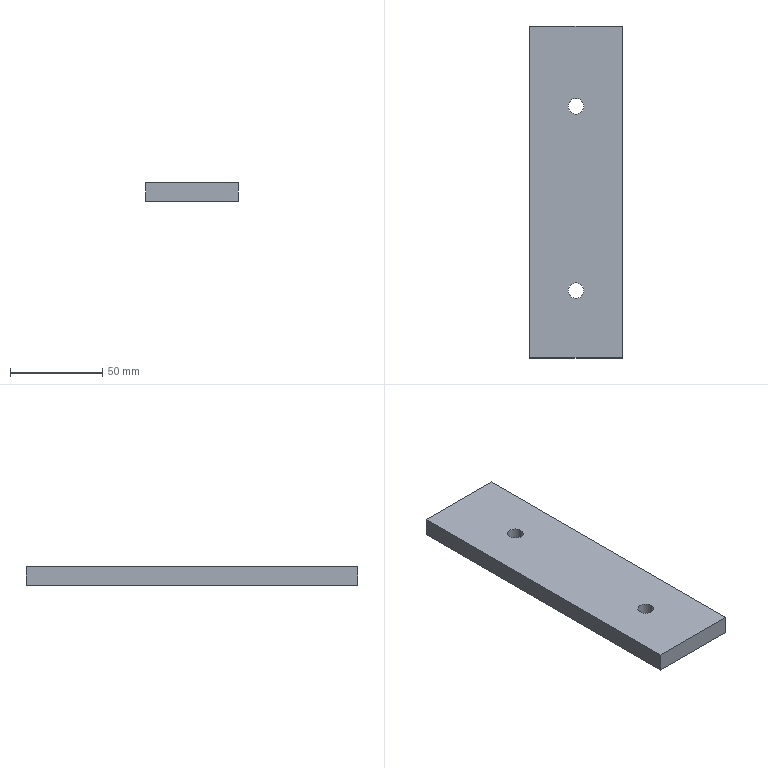Part | SolidWorks | features BaseBody 1, ICE 1 | 1 solid | 10 faces | box 50 x 180 x 10 mm | volume 88865 mm3 | plane 6 | cylinder 4 | commonest cylinder face diameters 8.5 x4
STEP:
#1=CARTESIAN_POINT('',(4.25,46.5,0.));
#2=VERTEX_POINT('',#1);
#3=CARTESIAN_POINT('',(-4.25,46.5,0.));
#4=VERTEX_POINT('',#3);
#5=CARTESIAN_POINT('',(0.,46.5,0.));
#6=DIRECTION('',(0.,0.,-1.));
#7=DIRECTION('',(1.,0.,0.));
#8=AXIS2_PLACEMENT_3D('',#5,#6,#7);
#9=CIRCLE('',#8,4.25);
#10=EDGE_CURVE('',#2,#4,#9,.T.);
#11=ORIENTED_EDGE('',*,*,#10,.T.);
#12=CARTESIAN_POINT('',(-4.25,46.5,10.));
#13=VERTEX_POINT('',#12);
#14=CARTESIAN_POINT('',(-4.25,46.5,-0.001));
#15=DIRECTION('',(0.,0.,1.));
#16=VECTOR('',#15,1000.);
#17=LINE('',#14,#16);
#18=EDGE_CURVE('',#4,#13,#17,.T.);
#19=ORIENTED_EDGE('',*,*,#18,.T.);
#20=CARTESIAN_POINT('',(4.25,46.5,10.));
#21=VERTEX_POINT('',#20);
#22=CARTESIAN_POINT('',(0.,46.5,10.));
#23=DIRECTION('',(0.,0.,1.));
#24=DIRECTION('',(1.,0.,0.));
#25=AXIS2_PLACEMENT_3D('',#22,#23,#24);
#26=CIRCLE('',#25,4.25);
#27=EDGE_CURVE('',#13,#21,#26,.T.);
#28=ORIENTED_EDGE('',*,*,#27,.T.);
#29=CARTESIAN_POINT('',(4.25,46.5,-0.001));
#30=DIRECTION('',(0.,0.,1.));
#31=VECTOR('',#30,1000.);
#32=LINE('',#29,#31);
#33=EDGE_CURVE('',#2,#21,#32,.T.);
#34=ORIENTED_EDGE('',*,*,#33,.F.);
#35=EDGE_LOOP('',(#11,#19,#28,#34));
#36=FACE_OUTER_BOUND('',#35,.T.);
#37=CARTESIAN_POINT('',(0.,46.5,-0.001));
#38=DIRECTION('',(0.,0.,1.));
#39=DIRECTION('',(1.,0.,0.));
#40=AXIS2_PLACEMENT_3D('',#37,#38,#39);
#41=CYLINDRICAL_SURFACE('',#40,4.25);
#42=ADVANCED_FACE('',(#36),#41,.F.);
#43=CARTESIAN_POINT('',(4.25,-53.5,0.));
#44=VERTEX_POINT('',#43);
#45=CARTESIAN_POINT('',(-4.25,-53.5,0.));
#46=VERTEX_POINT('',#45);
#47=CARTESIAN_POINT('',(0.,-53.5,0.));
#48=DIRECTION('',(0.,0.,-1.));
#49=DIRECTION('',(1.,0.,0.));
#50=AXIS2_PLACEMENT_3D('',#47,#48,#49);
#51=CIRCLE('',#50,4.25);
#52=EDGE_CURVE('',#44,#46,#51,.T.);
#53=ORIENTED_EDGE('',*,*,#52,.T.);
#54=CARTESIAN_POINT('',(-4.25,-53.5,10.));
#55=VERTEX_POINT('',#54);
#56=CARTESIAN_POINT('',(-4.25,-53.5,-0.001));
#57=DIRECTION('',(0.,0.,1.));
#58=VECTOR('',#57,1000.);
#59=LINE('',#56,#58);
#60=EDGE_CURVE('',#46,#55,#59,.T.);
#61=ORIENTED_EDGE('',*,*,#60,.T.);
#62=CARTESIAN_POINT('',(4.25,-53.5,10.));
#63=VERTEX_POINT('',#62);
#64=CARTESIAN_POINT('',(0.,-53.5,10.));
#65=DIRECTION('',(0.,0.,1.));
#66=DIRECTION('',(1.,0.,0.));
#67=AXIS2_PLACEMENT_3D('',#64,#65,#66);
#68=CIRCLE('',#67,4.25);
#69=EDGE_CURVE('',#55,#63,#68,.T.);
#70=ORIENTED_EDGE('',*,*,#69,.T.);
#71=CARTESIAN_POINT('',(4.25,-53.5,-0.001));
#72=DIRECTION('',(0.,0.,1.));
#73=VECTOR('',#72,1000.);
#74=LINE('',#71,#73);
#75=EDGE_CURVE('',#44,#63,#74,.T.);
#76=ORIENTED_EDGE('',*,*,#75,.F.);
#77=EDGE_LOOP('',(#53,#61,#70,#76));
#78=FACE_OUTER_BOUND('',#77,.T.);
#79=CARTESIAN_POINT('',(0.,-53.5,-0.001));
#80=DIRECTION('',(0.,0.,1.));
#81=DIRECTION('',(1.,0.,0.));
#82=AXIS2_PLACEMENT_3D('',#79,#80,#81);
#83=CYLINDRICAL_SURFACE('',#82,4.25);
#84=ADVANCED_FACE('',(#78),#83,.F.);
#85=ORIENTED_EDGE('',*,*,#10,.F.);
#86=CARTESIAN_POINT('',(0.,46.5,0.));
#87=DIRECTION('',(0.,0.,-1.));
#88=DIRECTION('',(1.,0.,0.));
#89=AXIS2_PLACEMENT_3D('',#86,#87,#88);
#90=CIRCLE('',#89,4.25);
#91=EDGE_CURVE('',#4,#2,#90,.T.);
#92=ORIENTED_EDGE('',*,*,#91,.F.);
#93=EDGE_LOOP('',(#85,#92));
#94=FACE_BOUND('',#93,.T.);
#95=ORIENTED_EDGE('',*,*,#52,.F.);
#96=CARTESIAN_POINT('',(0.,-53.5,0.));
#97=DIRECTION('',(0.,0.,-1.));
#98=DIRECTION('',(1.,0.,0.));
#99=AXIS2_PLACEMENT_3D('',#96,#97,#98);
#100=CIRCLE('',#99,4.25);
#101=EDGE_CURVE('',#46,#44,#100,.T.);
#102=ORIENTED_EDGE('',*,*,#101,.F.);
#103=EDGE_LOOP('',(#95,#102));
#104=FACE_BOUND('',#103,.T.);
#105=CARTESIAN_POINT('',(25.,-90.,0.));
#106=VERTEX_POINT('',#105);
#107=CARTESIAN_POINT('',(25.,90.,0.));
#108=VERTEX_POINT('',#107);
#109=CARTESIAN_POINT('',(25.,90.,0.));
#110=DIRECTION('',(0.,1.,0.));
#111=VECTOR('',#110,1000.);
#112=LINE('',#109,#111);
#113=EDGE_CURVE('',#106,#108,#112,.T.);
#114=ORIENTED_EDGE('',*,*,#113,.F.);
#115=CARTESIAN_POINT('',(-25.,-90.,0.));
#116=VERTEX_POINT('',#115);
#117=CARTESIAN_POINT('',(-25.,-90.,0.));
#118=DIRECTION('',(1.,0.,0.));
#119=VECTOR('',#118,1000.);
#120=LINE('',#117,#119);
#121=EDGE_CURVE('',#116,#106,#120,.T.);
#122=ORIENTED_EDGE('',*,*,#121,.F.);
#123=CARTESIAN_POINT('',(-25.,90.,0.));
#124=VERTEX_POINT('',#123);
#125=CARTESIAN_POINT('',(-25.,90.,0.));
#126=DIRECTION('',(0.,-1.,0.));
#127=VECTOR('',#126,1000.);
#128=LINE('',#125,#127);
#129=EDGE_CURVE('',#124,#116,#128,.T.);
#130=ORIENTED_EDGE('',*,*,#129,.F.);
#131=CARTESIAN_POINT('',(-25.,90.,0.));
#132=DIRECTION('',(-1.,0.,0.));
#133=VECTOR('',#132,1000.);
#134=LINE('',#131,#133);
#135=EDGE_CURVE('',#108,#124,#134,.T.);
#136=ORIENTED_EDGE('',*,*,#135,.F.);
#137=EDGE_LOOP('',(#114,#122,#130,#136));
#138=FACE_OUTER_BOUND('',#137,.T.);
#139=CARTESIAN_POINT('',(0.,0.,0.));
#140=DIRECTION('',(0.,0.,1.));
#141=DIRECTION('',(1.,0.,0.));
#142=AXIS2_PLACEMENT_3D('',#139,#140,#141);
#143=PLANE('',#142);
#144=ADVANCED_FACE('',(#94,#104,#138),#143,.F.);
#145=CARTESIAN_POINT('',(0.,46.5,10.));
#146=DIRECTION('',(0.,0.,1.));
#147=DIRECTION('',(1.,0.,0.));
#148=AXIS2_PLACEMENT_3D('',#145,#146,#147);
#149=CIRCLE('',#148,4.25);
#150=EDGE_CURVE('',#21,#13,#149,.T.);
#151=ORIENTED_EDGE('',*,*,#150,.F.);
#152=ORIENTED_EDGE('',*,*,#27,.F.);
#153=EDGE_LOOP('',(#151,#152));
#154=FACE_BOUND('',#153,.T.);
#155=CARTESIAN_POINT('',(0.,-53.5,10.));
#156=DIRECTION('',(0.,0.,1.));
#157=DIRECTION('',(1.,0.,0.));
#158=AXIS2_PLACEMENT_3D('',#155,#156,#157);
#159=CIRCLE('',#158,4.25);
#160=EDGE_CURVE('',#63,#55,#159,.T.);
#161=ORIENTED_EDGE('',*,*,#160,.F.);
#162=ORIENTED_EDGE('',*,*,#69,.F.);
#163=EDGE_LOOP('',(#161,#162));
#164=FACE_BOUND('',#163,.T.);
#165=CARTESIAN_POINT('',(25.,-90.,10.));
#166=VERTEX_POINT('',#165);
#167=CARTESIAN_POINT('',(25.,90.,10.));
#168=VERTEX_POINT('',#167);
#169=CARTESIAN_POINT('',(25.,90.,10.));
#170=DIRECTION('',(0.,1.,0.));
#171=VECTOR('',#170,1000.);
#172=LINE('',#169,#171);
#173=EDGE_CURVE('',#166,#168,#172,.T.);
#174=ORIENTED_EDGE('',*,*,#173,.T.);
#175=CARTESIAN_POINT('',(-25.,90.,10.));
#176=VERTEX_POINT('',#175);
#177=CARTESIAN_POINT('',(-25.,90.,10.));
#178=DIRECTION('',(-1.,0.,0.));
#179=VECTOR('',#178,1000.);
#180=LINE('',#177,#179);
#181=EDGE_CURVE('',#168,#176,#180,.T.);
#182=ORIENTED_EDGE('',*,*,#181,.T.);
#183=CARTESIAN_POINT('',(-25.,-90.,10.));
#184=VERTEX_POINT('',#183);
#185=CARTESIAN_POINT('',(-25.,90.,10.));
#186=DIRECTION('',(0.,-1.,0.));
#187=VECTOR('',#186,1000.);
#188=LINE('',#185,#187);
#189=EDGE_CURVE('',#176,#184,#188,.T.);
#190=ORIENTED_EDGE('',*,*,#189,.T.);
#191=CARTESIAN_POINT('',(-25.,-90.,10.));
#192=DIRECTION('',(1.,0.,0.));
#193=VECTOR('',#192,1000.);
#194=LINE('',#191,#193);
#195=EDGE_CURVE('',#184,#166,#194,.T.);
#196=ORIENTED_EDGE('',*,*,#195,.T.);
#197=EDGE_LOOP('',(#174,#182,#190,#196));
#198=FACE_OUTER_BOUND('',#197,.T.);
#199=CARTESIAN_POINT('',(0.,0.,10.));
#200=DIRECTION('',(0.,0.,1.));
#201=DIRECTION('',(1.,0.,0.));
#202=AXIS2_PLACEMENT_3D('',#199,#200,#201);
#203=PLANE('',#202);
#204=ADVANCED_FACE('',(#154,#164,#198),#203,.T.);
#205=ORIENTED_EDGE('',*,*,#121,.T.);
#206=CARTESIAN_POINT('',(25.,-90.,10.));
#207=DIRECTION('',(0.,0.,-1.));
#208=VECTOR('',#207,1000.);
#209=LINE('',#206,#208);
#210=EDGE_CURVE('',#166,#106,#209,.T.);
#211=ORIENTED_EDGE('',*,*,#210,.F.);
#212=ORIENTED_EDGE('',*,*,#195,.F.);
#213=CARTESIAN_POINT('',(-25.,-90.,10.));
#214=DIRECTION('',(0.,0.,-1.));
#215=VECTOR('',#214,1000.);
#216=LINE('',#213,#215);
#217=EDGE_CURVE('',#184,#116,#216,.T.);
#218=ORIENTED_EDGE('',*,*,#217,.T.);
#219=EDGE_LOOP('',(#205,#211,#212,#218));
#220=FACE_OUTER_BOUND('',#219,.T.);
#221=CARTESIAN_POINT('',(-25.,-90.,10.));
#222=DIRECTION('',(0.,1.,0.));
#223=DIRECTION('',(1.,0.,0.));
#224=AXIS2_PLACEMENT_3D('',#221,#222,#223);
#225=PLANE('',#224);
#226=ADVANCED_FACE('',(#220),#225,.F.);
#227=ORIENTED_EDGE('',*,*,#129,.T.);
#228=ORIENTED_EDGE('',*,*,#217,.F.);
#229=ORIENTED_EDGE('',*,*,#189,.F.);
#230=CARTESIAN_POINT('',(-25.,90.,10.));
#231=DIRECTION('',(0.,0.,-1.));
#232=VECTOR('',#231,1000.);
#233=LINE('',#230,#232);
#234=EDGE_CURVE('',#176,#124,#233,.T.);
#235=ORIENTED_EDGE('',*,*,#234,.T.);
#236=EDGE_LOOP('',(#227,#228,#229,#235));
#237=FACE_OUTER_BOUND('',#236,.T.);
#238=CARTESIAN_POINT('',(-25.,90.,10.));
#239=DIRECTION('',(1.,0.,0.));
#240=DIRECTION('',(0.,1.,0.));
#241=AXIS2_PLACEMENT_3D('',#238,#239,#240);
#242=PLANE('',#241);
#243=ADVANCED_FACE('',(#237),#242,.F.);
#244=ORIENTED_EDGE('',*,*,#135,.T.);
#245=ORIENTED_EDGE('',*,*,#234,.F.);
#246=ORIENTED_EDGE('',*,*,#181,.F.);
#247=CARTESIAN_POINT('',(25.,90.,10.));
#248=DIRECTION('',(0.,0.,-1.));
#249=VECTOR('',#248,1000.);
#250=LINE('',#247,#249);
#251=EDGE_CURVE('',#168,#108,#250,.T.);
#252=ORIENTED_EDGE('',*,*,#251,.T.);
#253=EDGE_LOOP('',(#244,#245,#246,#252));
#254=FACE_OUTER_BOUND('',#253,.T.);
#255=CARTESIAN_POINT('',(-25.,90.,10.));
#256=DIRECTION('',(0.,-1.,0.));
#257=DIRECTION('',(0.,0.,-1.));
#258=AXIS2_PLACEMENT_3D('',#255,#256,#257);
#259=PLANE('',#258);
#260=ADVANCED_FACE('',(#254),#259,.F.);
#261=ORIENTED_EDGE('',*,*,#113,.T.);
#262=ORIENTED_EDGE('',*,*,#251,.F.);
#263=ORIENTED_EDGE('',*,*,#173,.F.);
#264=ORIENTED_EDGE('',*,*,#210,.T.);
#265=EDGE_LOOP('',(#261,#262,#263,#264));
#266=FACE_OUTER_BOUND('',#265,.T.);
#267=CARTESIAN_POINT('',(25.,90.,10.));
#268=DIRECTION('',(-1.,0.,0.));
#269=DIRECTION('',(0.,1.,0.));
#270=AXIS2_PLACEMENT_3D('',#267,#268,#269);
#271=PLANE('',#270);
#272=ADVANCED_FACE('',(#266),#271,.F.);
#273=ORIENTED_EDGE('',*,*,#60,.F.);
#274=ORIENTED_EDGE('',*,*,#101,.T.);
#275=ORIENTED_EDGE('',*,*,#75,.T.);
#276=ORIENTED_EDGE('',*,*,#160,.T.);
#277=EDGE_LOOP('',(#273,#274,#275,#276));
#278=FACE_OUTER_BOUND('',#277,.T.);
#279=CARTESIAN_POINT('',(0.,-53.5,-0.001));
#280=DIRECTION('',(0.,0.,1.));
#281=DIRECTION('',(1.,0.,0.));
#282=AXIS2_PLACEMENT_3D('',#279,#280,#281);
#283=CYLINDRICAL_SURFACE('',#282,4.25);
#284=ADVANCED_FACE('',(#278),#283,.F.);
#285=ORIENTED_EDGE('',*,*,#18,.F.);
#286=ORIENTED_EDGE('',*,*,#91,.T.);
#287=ORIENTED_EDGE('',*,*,#33,.T.);
#288=ORIENTED_EDGE('',*,*,#150,.T.);
#289=EDGE_LOOP('',(#285,#286,#287,#288));
#290=FACE_OUTER_BOUND('',#289,.T.);
#291=CARTESIAN_POINT('',(0.,46.5,-0.001));
#292=DIRECTION('',(0.,0.,1.));
#293=DIRECTION('',(1.,0.,0.));
#294=AXIS2_PLACEMENT_3D('',#291,#292,#293);
#295=CYLINDRICAL_SURFACE('',#294,4.25);
#296=ADVANCED_FACE('',(#290),#295,.F.);
#297=CLOSED_SHELL('',(#42,#84,#144,#204,#226,#243,#260,#272,#284,#296));
#298=MANIFOLD_SOLID_BREP('',#297);
#299=CARTESIAN_POINT('',(0.,0.,0.));
#300=DIRECTION('',(0.,0.,1.));
#301=DIRECTION('',(1.,0.,0.));
#302=AXIS2_PLACEMENT_3D('',#299,#300,#301);
#303=(LENGTH_UNIT()NAMED_UNIT(*)SI_UNIT(.MILLI.,.METRE.));
#304=UNCERTAINTY_MEASURE_WITH_UNIT(LENGTH_MEASURE(0.00001),#303,'','');
#305=(NAMED_UNIT(*)PLANE_ANGLE_UNIT()SI_UNIT($,.RADIAN.));
#306=(NAMED_UNIT(*)SI_UNIT($,.STERADIAN.)SOLID_ANGLE_UNIT());
#307=(GEOMETRIC_REPRESENTATION_CONTEXT(3)GLOBAL_UNCERTAINTY_ASSIGNED_CONTEXT((#304))GLOBAL_UNIT_ASSIGNED_CONTEXT((#303,#305,#306))REPRESENTATION_CONTEXT('',''));
#308=ADVANCED_BREP_SHAPE_REPRESENTATION('',(#298,#302),#307);